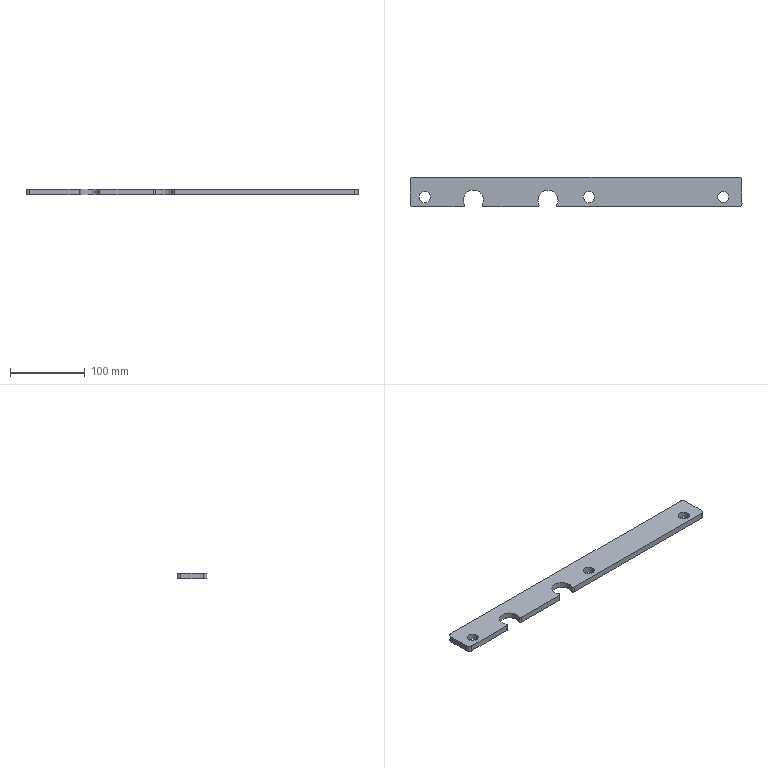Part | SolidWorks | features Fillet 1, FlatPattern 1, SMBaseFlange 1, SheetMetal 1 | 1 solid | 30 faces | box 445.22 x 40 x 8 mm | volume 129798 mm3 | cylinder 22 | plane 8 | commonest cylinder face diameters 4 x6 15 x6 27 x6 10 x4
STEP:
#1=CARTESIAN_POINT('',(-35.671,12.,8.));
#2=VERTEX_POINT('',#1);
#3=CARTESIAN_POINT('',(-33.671,10.,8.));
#4=VERTEX_POINT('',#3);
#5=CARTESIAN_POINT('',(-33.671,12.,8.));
#6=DIRECTION('',(0.,0.,1.));
#7=DIRECTION('',(1.,0.,0.));
#8=AXIS2_PLACEMENT_3D('',#5,#6,#7);
#9=CIRCLE('',#8,2.);
#10=EDGE_CURVE('',#2,#4,#9,.T.);
#11=ORIENTED_EDGE('',*,*,#10,.F.);
#12=CARTESIAN_POINT('',(-35.671,12.,0.));
#13=VERTEX_POINT('',#12);
#14=CARTESIAN_POINT('',(-35.671,12.,8.));
#15=DIRECTION('',(0.,0.,-1.));
#16=VECTOR('',#15,1000.);
#17=LINE('',#14,#16);
#18=EDGE_CURVE('',#2,#13,#17,.T.);
#19=ORIENTED_EDGE('',*,*,#18,.T.);
#20=CARTESIAN_POINT('',(-33.671,10.,0.));
#21=VERTEX_POINT('',#20);
#22=CARTESIAN_POINT('',(-33.671,12.,0.));
#23=DIRECTION('',(0.,0.,-1.));
#24=DIRECTION('',(1.,0.,0.));
#25=AXIS2_PLACEMENT_3D('',#22,#23,#24);
#26=CIRCLE('',#25,2.);
#27=EDGE_CURVE('',#21,#13,#26,.T.);
#28=ORIENTED_EDGE('',*,*,#27,.F.);
#29=CARTESIAN_POINT('',(-33.671,10.,8.));
#30=DIRECTION('',(0.,0.,-1.));
#31=VECTOR('',#30,1000.);
#32=LINE('',#29,#31);
#33=EDGE_CURVE('',#4,#21,#32,.T.);
#34=ORIENTED_EDGE('',*,*,#33,.F.);
#35=EDGE_LOOP('',(#11,#19,#28,#34));
#36=FACE_OUTER_BOUND('',#35,.T.);
#37=CARTESIAN_POINT('',(-33.671,12.,8.));
#38=DIRECTION('',(0.,0.,-1.));
#39=DIRECTION('',(-1.,0.,0.));
#40=AXIS2_PLACEMENT_3D('',#37,#38,#39);
#41=CYLINDRICAL_SURFACE('',#40,2.);
#42=ADVANCED_FACE('',(#36),#41,.T.);
#43=CARTESIAN_POINT('',(64.329,12.,8.));
#44=VERTEX_POINT('',#43);
#45=CARTESIAN_POINT('',(66.329,10.,8.));
#46=VERTEX_POINT('',#45);
#47=CARTESIAN_POINT('',(66.329,12.,8.));
#48=DIRECTION('',(0.,0.,1.));
#49=DIRECTION('',(1.,0.,0.));
#50=AXIS2_PLACEMENT_3D('',#47,#48,#49);
#51=CIRCLE('',#50,2.);
#52=EDGE_CURVE('',#44,#46,#51,.T.);
#53=ORIENTED_EDGE('',*,*,#52,.F.);
#54=CARTESIAN_POINT('',(64.329,12.,0.));
#55=VERTEX_POINT('',#54);
#56=CARTESIAN_POINT('',(64.329,12.,8.));
#57=DIRECTION('',(0.,0.,-1.));
#58=VECTOR('',#57,1000.);
#59=LINE('',#56,#58);
#60=EDGE_CURVE('',#44,#55,#59,.T.);
#61=ORIENTED_EDGE('',*,*,#60,.T.);
#62=CARTESIAN_POINT('',(66.329,10.,0.));
#63=VERTEX_POINT('',#62);
#64=CARTESIAN_POINT('',(66.329,12.,0.));
#65=DIRECTION('',(0.,0.,-1.));
#66=DIRECTION('',(1.,0.,0.));
#67=AXIS2_PLACEMENT_3D('',#64,#65,#66);
#68=CIRCLE('',#67,2.);
#69=EDGE_CURVE('',#63,#55,#68,.T.);
#70=ORIENTED_EDGE('',*,*,#69,.F.);
#71=CARTESIAN_POINT('',(66.329,10.,8.));
#72=DIRECTION('',(0.,0.,-1.));
#73=VECTOR('',#72,1000.);
#74=LINE('',#71,#73);
#75=EDGE_CURVE('',#46,#63,#74,.T.);
#76=ORIENTED_EDGE('',*,*,#75,.F.);
#77=EDGE_LOOP('',(#53,#61,#70,#76));
#78=FACE_OUTER_BOUND('',#77,.T.);
#79=CARTESIAN_POINT('',(66.329,12.,8.));
#80=DIRECTION('',(0.,0.,-1.));
#81=DIRECTION('',(-1.,0.,0.));
#82=AXIS2_PLACEMENT_3D('',#79,#80,#81);
#83=CYLINDRICAL_SURFACE('',#82,2.);
#84=ADVANCED_FACE('',(#78),#83,.T.);
#85=CARTESIAN_POINT('',(279.991,23.188,8.));
#86=VERTEX_POINT('',#85);
#87=CARTESIAN_POINT('',(294.991,23.188,8.));
#88=VERTEX_POINT('',#87);
#89=CARTESIAN_POINT('',(287.491,23.188,8.));
#90=DIRECTION('',(0.,0.,1.));
#91=DIRECTION('',(1.,0.,0.));
#92=AXIS2_PLACEMENT_3D('',#89,#90,#91);
#93=CIRCLE('',#92,7.5);
#94=EDGE_CURVE('',#86,#88,#93,.T.);
#95=ORIENTED_EDGE('',*,*,#94,.T.);
#96=CARTESIAN_POINT('',(294.991,23.188,0.));
#97=VERTEX_POINT('',#96);
#98=CARTESIAN_POINT('',(294.991,23.188,8.));
#99=DIRECTION('',(0.,0.,-1.));
#100=VECTOR('',#99,1000.);
#101=LINE('',#98,#100);
#102=EDGE_CURVE('',#88,#97,#101,.T.);
#103=ORIENTED_EDGE('',*,*,#102,.T.);
#104=CARTESIAN_POINT('',(279.991,23.188,0.));
#105=VERTEX_POINT('',#104);
#106=CARTESIAN_POINT('',(287.491,23.188,0.));
#107=DIRECTION('',(0.,0.,1.));
#108=DIRECTION('',(1.,0.,0.));
#109=AXIS2_PLACEMENT_3D('',#106,#107,#108);
#110=CIRCLE('',#109,7.5);
#111=EDGE_CURVE('',#105,#97,#110,.T.);
#112=ORIENTED_EDGE('',*,*,#111,.F.);
#113=CARTESIAN_POINT('',(279.991,23.188,8.));
#114=DIRECTION('',(0.,0.,-1.));
#115=VECTOR('',#114,1000.);
#116=LINE('',#113,#115);
#117=EDGE_CURVE('',#86,#105,#116,.T.);
#118=ORIENTED_EDGE('',*,*,#117,.F.);
#119=EDGE_LOOP('',(#95,#103,#112,#118));
#120=FACE_OUTER_BOUND('',#119,.T.);
#121=CARTESIAN_POINT('',(287.491,23.188,8.));
#122=DIRECTION('',(0.,0.,-1.));
#123=DIRECTION('',(-1.,0.,0.));
#124=AXIS2_PLACEMENT_3D('',#121,#122,#123);
#125=CYLINDRICAL_SURFACE('',#124,7.5);
#126=ADVANCED_FACE('',(#120),#125,.F.);
#127=CARTESIAN_POINT('',(100.,23.,8.));
#128=VERTEX_POINT('',#127);
#129=CARTESIAN_POINT('',(115.,23.,8.));
#130=VERTEX_POINT('',#129);
#131=CARTESIAN_POINT('',(107.5,23.,8.));
#132=DIRECTION('',(0.,0.,1.));
#133=DIRECTION('',(1.,0.,0.));
#134=AXIS2_PLACEMENT_3D('',#131,#132,#133);
#135=CIRCLE('',#134,7.5);
#136=EDGE_CURVE('',#128,#130,#135,.T.);
#137=ORIENTED_EDGE('',*,*,#136,.T.);
#138=CARTESIAN_POINT('',(115.,23.,0.));
#139=VERTEX_POINT('',#138);
#140=CARTESIAN_POINT('',(115.,23.,8.));
#141=DIRECTION('',(0.,0.,-1.));
#142=VECTOR('',#141,1000.);
#143=LINE('',#140,#142);
#144=EDGE_CURVE('',#130,#139,#143,.T.);
#145=ORIENTED_EDGE('',*,*,#144,.T.);
#146=CARTESIAN_POINT('',(100.,23.,0.));
#147=VERTEX_POINT('',#146);
#148=CARTESIAN_POINT('',(107.5,23.,0.));
#149=DIRECTION('',(0.,0.,1.));
#150=DIRECTION('',(1.,0.,0.));
#151=AXIS2_PLACEMENT_3D('',#148,#149,#150);
#152=CIRCLE('',#151,7.5);
#153=EDGE_CURVE('',#147,#139,#152,.T.);
#154=ORIENTED_EDGE('',*,*,#153,.F.);
#155=CARTESIAN_POINT('',(100.,23.,8.));
#156=DIRECTION('',(0.,0.,-1.));
#157=VECTOR('',#156,1000.);
#158=LINE('',#155,#157);
#159=EDGE_CURVE('',#128,#147,#158,.T.);
#160=ORIENTED_EDGE('',*,*,#159,.F.);
#161=EDGE_LOOP('',(#137,#145,#154,#160));
#162=FACE_OUTER_BOUND('',#161,.T.);
#163=CARTESIAN_POINT('',(107.5,23.,8.));
#164=DIRECTION('',(0.,0.,-1.));
#165=DIRECTION('',(-1.,0.,0.));
#166=AXIS2_PLACEMENT_3D('',#163,#164,#165);
#167=CYLINDRICAL_SURFACE('',#166,7.5);
#168=ADVANCED_FACE('',(#162),#167,.F.);
#169=CARTESIAN_POINT('',(-120.,23.,8.));
#170=VERTEX_POINT('',#169);
#171=CARTESIAN_POINT('',(-105.,23.,8.));
#172=VERTEX_POINT('',#171);
#173=CARTESIAN_POINT('',(-112.5,23.,8.));
#174=DIRECTION('',(0.,0.,1.));
#175=DIRECTION('',(1.,0.,0.));
#176=AXIS2_PLACEMENT_3D('',#173,#174,#175);
#177=CIRCLE('',#176,7.5);
#178=EDGE_CURVE('',#170,#172,#177,.T.);
#179=ORIENTED_EDGE('',*,*,#178,.T.);
#180=CARTESIAN_POINT('',(-105.,23.,0.));
#181=VERTEX_POINT('',#180);
#182=CARTESIAN_POINT('',(-105.,23.,8.));
#183=DIRECTION('',(0.,0.,-1.));
#184=VECTOR('',#183,1000.);
#185=LINE('',#182,#184);
#186=EDGE_CURVE('',#172,#181,#185,.T.);
#187=ORIENTED_EDGE('',*,*,#186,.T.);
#188=CARTESIAN_POINT('',(-120.,23.,0.));
#189=VERTEX_POINT('',#188);
#190=CARTESIAN_POINT('',(-112.5,23.,0.));
#191=DIRECTION('',(0.,0.,1.));
#192=DIRECTION('',(1.,0.,0.));
#193=AXIS2_PLACEMENT_3D('',#190,#191,#192);
#194=CIRCLE('',#193,7.5);
#195=EDGE_CURVE('',#189,#181,#194,.T.);
#196=ORIENTED_EDGE('',*,*,#195,.F.);
#197=CARTESIAN_POINT('',(-120.,23.,8.));
#198=DIRECTION('',(0.,0.,-1.));
#199=VECTOR('',#198,1000.);
#200=LINE('',#197,#199);
#201=EDGE_CURVE('',#170,#189,#200,.T.);
#202=ORIENTED_EDGE('',*,*,#201,.F.);
#203=EDGE_LOOP('',(#179,#187,#196,#202));
#204=FACE_OUTER_BOUND('',#203,.T.);
#205=CARTESIAN_POINT('',(-112.5,23.,8.));
#206=DIRECTION('',(0.,0.,-1.));
#207=DIRECTION('',(-1.,0.,0.));
#208=AXIS2_PLACEMENT_3D('',#205,#206,#207);
#209=CYLINDRICAL_SURFACE('',#208,7.5);
#210=ADVANCED_FACE('',(#204),#209,.F.);
#211=CARTESIAN_POINT('',(66.,19.,8.));
#212=VERTEX_POINT('',#211);
#213=CARTESIAN_POINT('',(64.545,12.903,8.));
#214=VERTEX_POINT('',#213);
#215=CARTESIAN_POINT('',(52.5,19.,8.));
#216=DIRECTION('',(0.,0.,-1.));
#217=DIRECTION('',(1.,0.,0.));
#218=AXIS2_PLACEMENT_3D('',#215,#216,#217);
#219=CIRCLE('',#218,13.5);
#220=EDGE_CURVE('',#212,#214,#219,.T.);
#221=ORIENTED_EDGE('',*,*,#220,.F.);
#222=CARTESIAN_POINT('',(66.,19.,0.));
#223=VERTEX_POINT('',#222);
#224=CARTESIAN_POINT('',(66.,19.,8.));
#225=DIRECTION('',(0.,0.,-1.));
#226=VECTOR('',#225,1000.);
#227=LINE('',#224,#226);
#228=EDGE_CURVE('',#212,#223,#227,.T.);
#229=ORIENTED_EDGE('',*,*,#228,.T.);
#230=CARTESIAN_POINT('',(64.545,12.903,0.));
#231=VERTEX_POINT('',#230);
#232=CARTESIAN_POINT('',(52.5,19.,0.));
#233=DIRECTION('',(0.,0.,-1.));
#234=DIRECTION('',(1.,0.,0.));
#235=AXIS2_PLACEMENT_3D('',#232,#233,#234);
#236=CIRCLE('',#235,13.5);
#237=EDGE_CURVE('',#223,#231,#236,.T.);
#238=ORIENTED_EDGE('',*,*,#237,.T.);
#239=CARTESIAN_POINT('',(64.545,12.903,8.));
#240=DIRECTION('',(0.,0.,1.));
#241=VECTOR('',#240,1000.);
#242=LINE('',#239,#241);
#243=EDGE_CURVE('',#231,#214,#242,.T.);
#244=ORIENTED_EDGE('',*,*,#243,.T.);
#245=EDGE_LOOP('',(#221,#229,#238,#244));
#246=FACE_OUTER_BOUND('',#245,.T.);
#247=CARTESIAN_POINT('',(52.5,19.,8.));
#248=DIRECTION('',(0.,0.,-1.));
#249=DIRECTION('',(-1.,0.,0.));
#250=AXIS2_PLACEMENT_3D('',#247,#248,#249);
#251=CYLINDRICAL_SURFACE('',#250,13.5);
#252=ADVANCED_FACE('',(#246),#251,.F.);
#253=ORIENTED_EDGE('',*,*,#228,.F.);
#254=CARTESIAN_POINT('',(39.,19.,8.));
#255=VERTEX_POINT('',#254);
#256=CARTESIAN_POINT('',(52.5,19.,8.));
#257=DIRECTION('',(0.,0.,-1.));
#258=DIRECTION('',(1.,0.,0.));
#259=AXIS2_PLACEMENT_3D('',#256,#257,#258);
#260=CIRCLE('',#259,13.5);
#261=EDGE_CURVE('',#255,#212,#260,.T.);
#262=ORIENTED_EDGE('',*,*,#261,.F.);
#263=CARTESIAN_POINT('',(39.,19.,0.));
#264=VERTEX_POINT('',#263);
#265=CARTESIAN_POINT('',(39.,19.,8.));
#266=DIRECTION('',(0.,0.,-1.));
#267=VECTOR('',#266,1000.);
#268=LINE('',#265,#267);
#269=EDGE_CURVE('',#255,#264,#268,.T.);
#270=ORIENTED_EDGE('',*,*,#269,.T.);
#271=CARTESIAN_POINT('',(52.5,19.,0.));
#272=DIRECTION('',(0.,0.,-1.));
#273=DIRECTION('',(1.,0.,0.));
#274=AXIS2_PLACEMENT_3D('',#271,#272,#273);
#275=CIRCLE('',#274,13.5);
#276=EDGE_CURVE('',#264,#223,#275,.T.);
#277=ORIENTED_EDGE('',*,*,#276,.T.);
#278=EDGE_LOOP('',(#253,#262,#270,#277));
#279=FACE_OUTER_BOUND('',#278,.T.);
#280=CARTESIAN_POINT('',(52.5,19.,8.));
#281=DIRECTION('',(0.,0.,-1.));
#282=DIRECTION('',(-1.,0.,0.));
#283=AXIS2_PLACEMENT_3D('',#280,#281,#282);
#284=CYLINDRICAL_SURFACE('',#283,13.5);
#285=ADVANCED_FACE('',(#279),#284,.F.);
#286=CARTESIAN_POINT('',(-34.,19.,8.));
#287=VERTEX_POINT('',#286);
#288=CARTESIAN_POINT('',(-35.455,12.903,8.));
#289=VERTEX_POINT('',#288);
#290=CARTESIAN_POINT('',(-47.5,19.,8.));
#291=DIRECTION('',(0.,0.,-1.));
#292=DIRECTION('',(1.,0.,0.));
#293=AXIS2_PLACEMENT_3D('',#290,#291,#292);
#294=CIRCLE('',#293,13.5);
#295=EDGE_CURVE('',#287,#289,#294,.T.);
#296=ORIENTED_EDGE('',*,*,#295,.F.);
#297=CARTESIAN_POINT('',(-34.,19.,0.));
#298=VERTEX_POINT('',#297);
#299=CARTESIAN_POINT('',(-34.,19.,8.));
#300=DIRECTION('',(0.,0.,-1.));
#301=VECTOR('',#300,1000.);
#302=LINE('',#299,#301);
#303=EDGE_CURVE('',#287,#298,#302,.T.);
#304=ORIENTED_EDGE('',*,*,#303,.T.);
#305=CARTESIAN_POINT('',(-35.455,12.903,0.));
#306=VERTEX_POINT('',#305);
#307=CARTESIAN_POINT('',(-47.5,19.,0.));
#308=DIRECTION('',(0.,0.,-1.));
#309=DIRECTION('',(1.,0.,0.));
#310=AXIS2_PLACEMENT_3D('',#307,#308,#309);
#311=CIRCLE('',#310,13.5);
#312=EDGE_CURVE('',#298,#306,#311,.T.);
#313=ORIENTED_EDGE('',*,*,#312,.T.);
#314=CARTESIAN_POINT('',(-35.455,12.903,8.));
#315=DIRECTION('',(0.,0.,1.));
#316=VECTOR('',#315,1000.);
#317=LINE('',#314,#316);
#318=EDGE_CURVE('',#306,#289,#317,.T.);
#319=ORIENTED_EDGE('',*,*,#318,.T.);
#320=EDGE_LOOP('',(#296,#304,#313,#319));
#321=FACE_OUTER_BOUND('',#320,.T.);
#322=CARTESIAN_POINT('',(-47.5,19.,8.));
#323=DIRECTION('',(0.,0.,-1.));
#324=DIRECTION('',(-1.,0.,0.));
#325=AXIS2_PLACEMENT_3D('',#322,#323,#324);
#326=CYLINDRICAL_SURFACE('',#325,13.5);
#327=ADVANCED_FACE('',(#321),#326,.F.);
#328=ORIENTED_EDGE('',*,*,#303,.F.);
#329=CARTESIAN_POINT('',(-61.,19.,8.));
#330=VERTEX_POINT('',#329);
#331=CARTESIAN_POINT('',(-47.5,19.,8.));
#332=DIRECTION('',(0.,0.,-1.));
#333=DIRECTION('',(1.,0.,0.));
#334=AXIS2_PLACEMENT_3D('',#331,#332,#333);
#335=CIRCLE('',#334,13.5);
#336=EDGE_CURVE('',#330,#287,#335,.T.);
#337=ORIENTED_EDGE('',*,*,#336,.F.);
#338=CARTESIAN_POINT('',(-61.,19.,0.));
#339=VERTEX_POINT('',#338);
#340=CARTESIAN_POINT('',(-61.,19.,8.));
#341=DIRECTION('',(0.,0.,-1.));
#342=VECTOR('',#341,1000.);
#343=LINE('',#340,#342);
#344=EDGE_CURVE('',#330,#339,#343,.T.);
#345=ORIENTED_EDGE('',*,*,#344,.T.);
#346=CARTESIAN_POINT('',(-47.5,19.,0.));
#347=DIRECTION('',(0.,0.,-1.));
#348=DIRECTION('',(1.,0.,0.));
#349=AXIS2_PLACEMENT_3D('',#346,#347,#348);
#350=CIRCLE('',#349,13.5);
#351=EDGE_CURVE('',#339,#298,#350,.T.);
#352=ORIENTED_EDGE('',*,*,#351,.T.);
#353=EDGE_LOOP('',(#328,#337,#345,#352));
#354=FACE_OUTER_BOUND('',#353,.T.);
#355=CARTESIAN_POINT('',(-47.5,19.,8.));
#356=DIRECTION('',(0.,0.,-1.));
#357=DIRECTION('',(-1.,0.,0.));
#358=AXIS2_PLACEMENT_3D('',#355,#356,#357);
#359=CYLINDRICAL_SURFACE('',#358,13.5);
#360=ADVANCED_FACE('',(#354),#359,.F.);
#361=ORIENTED_EDGE('',*,*,#136,.F.);
#362=CARTESIAN_POINT('',(107.5,23.,8.));
#363=DIRECTION('',(0.,0.,1.));
#364=DIRECTION('',(1.,0.,0.));
#365=AXIS2_PLACEMENT_3D('',#362,#363,#364);
#366=CIRCLE('',#365,7.5);
#367=EDGE_CURVE('',#130,#128,#366,.T.);
#368=ORIENTED_EDGE('',*,*,#367,.F.);
#369=EDGE_LOOP('',(#361,#368));
#370=FACE_BOUND('',#369,.T.);
#371=CARTESIAN_POINT('',(38.671,10.,8.));
#372=VERTEX_POINT('',#371);
#373=CARTESIAN_POINT('',(42.438,10.,8.));
#374=DIRECTION('',(1.,0.,0.));
#375=VECTOR('',#374,1000.);
#376=LINE('',#373,#375);
#377=EDGE_CURVE('',#4,#372,#376,.T.);
#378=ORIENTED_EDGE('',*,*,#377,.T.);
#379=CARTESIAN_POINT('',(40.455,12.903,8.));
#380=VERTEX_POINT('',#379);
#381=CARTESIAN_POINT('',(38.671,12.,8.));
#382=DIRECTION('',(0.,0.,1.));
#383=DIRECTION('',(1.,0.,0.));
#384=AXIS2_PLACEMENT_3D('',#381,#382,#383);
#385=CIRCLE('',#384,2.);
#386=EDGE_CURVE('',#372,#380,#385,.T.);
#387=ORIENTED_EDGE('',*,*,#386,.T.);
#388=CARTESIAN_POINT('',(52.5,19.,8.));
#389=DIRECTION('',(0.,0.,-1.));
#390=DIRECTION('',(1.,0.,0.));
#391=AXIS2_PLACEMENT_3D('',#388,#389,#390);
#392=CIRCLE('',#391,13.5);
#393=EDGE_CURVE('',#380,#255,#392,.T.);
#394=ORIENTED_EDGE('',*,*,#393,.T.);
#395=ORIENTED_EDGE('',*,*,#261,.T.);
#396=ORIENTED_EDGE('',*,*,#220,.T.);
#397=CARTESIAN_POINT('',(66.329,12.,8.));
#398=DIRECTION('',(0.,0.,1.));
#399=DIRECTION('',(1.,0.,0.));
#400=AXIS2_PLACEMENT_3D('',#397,#398,#399);
#401=CIRCLE('',#400,2.);
#402=EDGE_CURVE('',#214,#44,#401,.T.);
#403=ORIENTED_EDGE('',*,*,#402,.T.);
#404=ORIENTED_EDGE('',*,*,#52,.T.);
#405=CARTESIAN_POINT('',(307.72,10.,8.));
#406=VERTEX_POINT('',#405);
#407=CARTESIAN_POINT('',(307.72,10.,8.));
#408=DIRECTION('',(1.,0.,0.));
#409=VECTOR('',#408,1000.);
#410=LINE('',#407,#409);
#411=EDGE_CURVE('',#46,#406,#410,.T.);
#412=ORIENTED_EDGE('',*,*,#411,.T.);
#413=CARTESIAN_POINT('',(312.72,15.01,8.));
#414=VERTEX_POINT('',#413);
#415=CARTESIAN_POINT('',(307.72,15.,8.));
#416=DIRECTION('',(0.,0.,1.));
#417=DIRECTION('',(-1.,0.,0.));
#418=AXIS2_PLACEMENT_3D('',#415,#416,#417);
#419=CIRCLE('',#418,5.);
#420=EDGE_CURVE('',#406,#414,#419,.T.);
#421=ORIENTED_EDGE('',*,*,#420,.T.);
#422=CARTESIAN_POINT('',(312.661,45.01,8.));
#423=VERTEX_POINT('',#422);
#424=CARTESIAN_POINT('',(312.661,45.01,8.));
#425=DIRECTION('',(-0.001974,1.,0.));
#426=VECTOR('',#425,1000.);
#427=LINE('',#424,#426);
#428=EDGE_CURVE('',#414,#423,#427,.T.);
#429=ORIENTED_EDGE('',*,*,#428,.T.);
#430=CARTESIAN_POINT('',(307.661,50.,8.));
#431=VERTEX_POINT('',#430);
#432=CARTESIAN_POINT('',(307.661,45.,8.));
#433=DIRECTION('',(0.,0.,1.));
#434=DIRECTION('',(-1.,0.,0.));
#435=AXIS2_PLACEMENT_3D('',#432,#433,#434);
#436=CIRCLE('',#435,5.);
#437=EDGE_CURVE('',#423,#431,#436,.T.);
#438=ORIENTED_EDGE('',*,*,#437,.T.);
#439=CARTESIAN_POINT('',(-127.5,50.,8.));
#440=VERTEX_POINT('',#439);
#441=CARTESIAN_POINT('',(-127.5,50.,8.));
#442=DIRECTION('',(-1.,0.,0.));
#443=VECTOR('',#442,1000.);
#444=LINE('',#441,#443);
#445=EDGE_CURVE('',#431,#440,#444,.T.);
#446=ORIENTED_EDGE('',*,*,#445,.T.);
#447=CARTESIAN_POINT('',(-132.5,45.,8.));
#448=VERTEX_POINT('',#447);
#449=CARTESIAN_POINT('',(-127.5,45.,8.));
#450=DIRECTION('',(0.,0.,1.));
#451=DIRECTION('',(-1.,0.,0.));
#452=AXIS2_PLACEMENT_3D('',#449,#450,#451);
#453=CIRCLE('',#452,5.);
#454=EDGE_CURVE('',#440,#448,#453,.T.);
#455=ORIENTED_EDGE('',*,*,#454,.T.);
#456=CARTESIAN_POINT('',(-132.5,15.,8.));
#457=VERTEX_POINT('',#456);
#458=CARTESIAN_POINT('',(-132.5,15.,8.));
#459=DIRECTION('',(0.,-1.,0.));
#460=VECTOR('',#459,1000.);
#461=LINE('',#458,#460);
#462=EDGE_CURVE('',#448,#457,#461,.T.);
#463=ORIENTED_EDGE('',*,*,#462,.T.);
#464=CARTESIAN_POINT('',(-127.5,10.,8.));
#465=VERTEX_POINT('',#464);
#466=CARTESIAN_POINT('',(-127.5,15.,8.));
#467=DIRECTION('',(0.,0.,1.));
#468=DIRECTION('',(1.,0.,0.));
#469=AXIS2_PLACEMENT_3D('',#466,#467,#468);
#470=CIRCLE('',#469,5.);
#471=EDGE_CURVE('',#457,#465,#470,.T.);
#472=ORIENTED_EDGE('',*,*,#471,.T.);
#473=CARTESIAN_POINT('',(-61.329,10.,8.));
#474=VERTEX_POINT('',#473);
#475=CARTESIAN_POINT('',(-57.562,10.,8.));
#476=DIRECTION('',(1.,0.,0.));
#477=VECTOR('',#476,1000.);
#478=LINE('',#475,#477);
#479=EDGE_CURVE('',#465,#474,#478,.T.);
#480=ORIENTED_EDGE('',*,*,#479,.T.);
#481=CARTESIAN_POINT('',(-59.545,12.903,8.));
#482=VERTEX_POINT('',#481);
#483=CARTESIAN_POINT('',(-61.329,12.,8.));
#484=DIRECTION('',(0.,0.,1.));
#485=DIRECTION('',(1.,0.,0.));
#486=AXIS2_PLACEMENT_3D('',#483,#484,#485);
#487=CIRCLE('',#486,2.);
#488=EDGE_CURVE('',#474,#482,#487,.T.);
#489=ORIENTED_EDGE('',*,*,#488,.T.);
#490=CARTESIAN_POINT('',(-47.5,19.,8.));
#491=DIRECTION('',(0.,0.,-1.));
#492=DIRECTION('',(1.,0.,0.));
#493=AXIS2_PLACEMENT_3D('',#490,#491,#492);
#494=CIRCLE('',#493,13.5);
#495=EDGE_CURVE('',#482,#330,#494,.T.);
#496=ORIENTED_EDGE('',*,*,#495,.T.);
#497=ORIENTED_EDGE('',*,*,#336,.T.);
#498=ORIENTED_EDGE('',*,*,#295,.T.);
#499=CARTESIAN_POINT('',(-33.671,12.,8.));
#500=DIRECTION('',(0.,0.,1.));
#501=DIRECTION('',(1.,0.,0.));
#502=AXIS2_PLACEMENT_3D('',#499,#500,#501);
#503=CIRCLE('',#502,2.);
#504=EDGE_CURVE('',#289,#2,#503,.T.);
#505=ORIENTED_EDGE('',*,*,#504,.T.);
#506=ORIENTED_EDGE('',*,*,#10,.T.);
#507=EDGE_LOOP('',(#378,#387,#394,#395,#396,#403,#404,#412,#421,#429,#438,#446,#455,#463,#472,#480,#489,#496,#497,#498,#505,#506));
#508=FACE_OUTER_BOUND('',#507,.T.);
#509=ORIENTED_EDGE('',*,*,#178,.F.);
#510=CARTESIAN_POINT('',(-112.5,23.,8.));
#511=DIRECTION('',(0.,0.,1.));
#512=DIRECTION('',(1.,0.,0.));
#513=AXIS2_PLACEMENT_3D('',#510,#511,#512);
#514=CIRCLE('',#513,7.5);
#515=EDGE_CURVE('',#172,#170,#514,.T.);
#516=ORIENTED_EDGE('',*,*,#515,.F.);
#517=EDGE_LOOP('',(#509,#516));
#518=FACE_BOUND('',#517,.T.);
#519=ORIENTED_EDGE('',*,*,#94,.F.);
#520=CARTESIAN_POINT('',(287.491,23.188,8.));
#521=DIRECTION('',(0.,0.,1.));
#522=DIRECTION('',(1.,0.,0.));
#523=AXIS2_PLACEMENT_3D('',#520,#521,#522);
#524=CIRCLE('',#523,7.5);
#525=EDGE_CURVE('',#88,#86,#524,.T.);
#526=ORIENTED_EDGE('',*,*,#525,.F.);
#527=EDGE_LOOP('',(#519,#526));
#528=FACE_BOUND('',#527,.T.);
#529=CARTESIAN_POINT('',(-47.5,19.,8.));
#530=DIRECTION('',(0.,0.,1.));
#531=DIRECTION('',(1.,0.,0.));
#532=AXIS2_PLACEMENT_3D('',#529,#530,#531);
#533=PLANE('',#532);
#534=ADVANCED_FACE('',(#370,#508,#518,#528),#533,.T.);
#535=CARTESIAN_POINT('',(40.455,12.903,0.));
#536=VERTEX_POINT('',#535);
#537=CARTESIAN_POINT('',(52.5,19.,0.));
#538=DIRECTION('',(0.,0.,-1.));
#539=DIRECTION('',(1.,0.,0.));
#540=AXIS2_PLACEMENT_3D('',#537,#538,#539);
#541=CIRCLE('',#540,13.5);
#542=EDGE_CURVE('',#536,#264,#541,.T.);
#543=ORIENTED_EDGE('',*,*,#542,.F.);
#544=CARTESIAN_POINT('',(38.671,10.,0.));
#545=VERTEX_POINT('',#544);
#546=CARTESIAN_POINT('',(38.671,12.,0.));
#547=DIRECTION('',(0.,0.,-1.));
#548=DIRECTION('',(1.,0.,0.));
#549=AXIS2_PLACEMENT_3D('',#546,#547,#548);
#550=CIRCLE('',#549,2.);
#551=EDGE_CURVE('',#536,#545,#550,.T.);
#552=ORIENTED_EDGE('',*,*,#551,.T.);
#553=CARTESIAN_POINT('',(42.438,10.,0.));
#554=DIRECTION('',(1.,0.,0.));
#555=VECTOR('',#554,1000.);
#556=LINE('',#553,#555);
#557=EDGE_CURVE('',#21,#545,#556,.T.);
#558=ORIENTED_EDGE('',*,*,#557,.F.);
#559=ORIENTED_EDGE('',*,*,#27,.T.);
#560=CARTESIAN_POINT('',(-33.671,12.,0.));
#561=DIRECTION('',(0.,0.,-1.));
#562=DIRECTION('',(1.,0.,0.));
#563=AXIS2_PLACEMENT_3D('',#560,#561,#562);
#564=CIRCLE('',#563,2.);
#565=EDGE_CURVE('',#13,#306,#564,.T.);
#566=ORIENTED_EDGE('',*,*,#565,.T.);
#567=ORIENTED_EDGE('',*,*,#312,.F.);
#568=ORIENTED_EDGE('',*,*,#351,.F.);
#569=CARTESIAN_POINT('',(-59.545,12.903,0.));
#570=VERTEX_POINT('',#569);
#571=CARTESIAN_POINT('',(-47.5,19.,0.));
#572=DIRECTION('',(0.,0.,-1.));
#573=DIRECTION('',(1.,0.,0.));
#574=AXIS2_PLACEMENT_3D('',#571,#572,#573);
#575=CIRCLE('',#574,13.5);
#576=EDGE_CURVE('',#570,#339,#575,.T.);
#577=ORIENTED_EDGE('',*,*,#576,.F.);
#578=CARTESIAN_POINT('',(-61.329,10.,0.));
#579=VERTEX_POINT('',#578);
#580=CARTESIAN_POINT('',(-61.329,12.,0.));
#581=DIRECTION('',(0.,0.,-1.));
#582=DIRECTION('',(1.,0.,0.));
#583=AXIS2_PLACEMENT_3D('',#580,#581,#582);
#584=CIRCLE('',#583,2.);
#585=EDGE_CURVE('',#570,#579,#584,.T.);
#586=ORIENTED_EDGE('',*,*,#585,.T.);
#587=CARTESIAN_POINT('',(-127.5,10.,0.));
#588=VERTEX_POINT('',#587);
#589=CARTESIAN_POINT('',(-57.562,10.,0.));
#590=DIRECTION('',(1.,0.,0.));
#591=VECTOR('',#590,1000.);
#592=LINE('',#589,#591);
#593=EDGE_CURVE('',#588,#579,#592,.T.);
#594=ORIENTED_EDGE('',*,*,#593,.F.);
#595=CARTESIAN_POINT('',(-132.5,15.,0.));
#596=VERTEX_POINT('',#595);
#597=CARTESIAN_POINT('',(-127.5,15.,0.));
#598=DIRECTION('',(0.,0.,1.));
#599=DIRECTION('',(1.,0.,0.));
#600=AXIS2_PLACEMENT_3D('',#597,#598,#599);
#601=CIRCLE('',#600,5.);
#602=EDGE_CURVE('',#596,#588,#601,.T.);
#603=ORIENTED_EDGE('',*,*,#602,.F.);
#604=CARTESIAN_POINT('',(-132.5,45.,0.));
#605=VERTEX_POINT('',#604);
#606=CARTESIAN_POINT('',(-132.5,15.,0.));
#607=DIRECTION('',(0.,-1.,0.));
#608=VECTOR('',#607,1000.);
#609=LINE('',#606,#608);
#610=EDGE_CURVE('',#605,#596,#609,.T.);
#611=ORIENTED_EDGE('',*,*,#610,.F.);
#612=CARTESIAN_POINT('',(-127.5,50.,0.));
#613=VERTEX_POINT('',#612);
#614=CARTESIAN_POINT('',(-127.5,45.,0.));
#615=DIRECTION('',(0.,0.,1.));
#616=DIRECTION('',(-1.,0.,0.));
#617=AXIS2_PLACEMENT_3D('',#614,#615,#616);
#618=CIRCLE('',#617,5.);
#619=EDGE_CURVE('',#613,#605,#618,.T.);
#620=ORIENTED_EDGE('',*,*,#619,.F.);
#621=CARTESIAN_POINT('',(307.661,50.,0.));
#622=VERTEX_POINT('',#621);
#623=CARTESIAN_POINT('',(-127.5,50.,0.));
#624=DIRECTION('',(-1.,0.,0.));
#625=VECTOR('',#624,1000.);
#626=LINE('',#623,#625);
#627=EDGE_CURVE('',#622,#613,#626,.T.);
#628=ORIENTED_EDGE('',*,*,#627,.F.);
#629=CARTESIAN_POINT('',(312.661,45.01,0.));
#630=VERTEX_POINT('',#629);
#631=CARTESIAN_POINT('',(307.661,45.,0.));
#632=DIRECTION('',(0.,0.,1.));
#633=DIRECTION('',(-1.,0.,0.));
#634=AXIS2_PLACEMENT_3D('',#631,#632,#633);
#635=CIRCLE('',#634,5.);
#636=EDGE_CURVE('',#630,#622,#635,.T.);
#637=ORIENTED_EDGE('',*,*,#636,.F.);
#638=CARTESIAN_POINT('',(312.72,15.01,0.));
#639=VERTEX_POINT('',#638);
#640=CARTESIAN_POINT('',(312.661,45.01,0.));
#641=DIRECTION('',(-0.001974,1.,0.));
#642=VECTOR('',#641,1000.);
#643=LINE('',#640,#642);
#644=EDGE_CURVE('',#639,#630,#643,.T.);
#645=ORIENTED_EDGE('',*,*,#644,.F.);
#646=CARTESIAN_POINT('',(307.72,10.,0.));
#647=VERTEX_POINT('',#646);
#648=CARTESIAN_POINT('',(307.72,15.,0.));
#649=DIRECTION('',(0.,0.,1.));
#650=DIRECTION('',(-1.,0.,0.));
#651=AXIS2_PLACEMENT_3D('',#648,#649,#650);
#652=CIRCLE('',#651,5.);
#653=EDGE_CURVE('',#647,#639,#652,.T.);
#654=ORIENTED_EDGE('',*,*,#653,.F.);
#655=CARTESIAN_POINT('',(307.72,10.,0.));
#656=DIRECTION('',(1.,0.,0.));
#657=VECTOR('',#656,1000.);
#658=LINE('',#655,#657);
#659=EDGE_CURVE('',#63,#647,#658,.T.);
#660=ORIENTED_EDGE('',*,*,#659,.F.);
#661=ORIENTED_EDGE('',*,*,#69,.T.);
#662=CARTESIAN_POINT('',(66.329,12.,0.));
#663=DIRECTION('',(0.,0.,-1.));
#664=DIRECTION('',(1.,0.,0.));
#665=AXIS2_PLACEMENT_3D('',#662,#663,#664);
#666=CIRCLE('',#665,2.);
#667=EDGE_CURVE('',#55,#231,#666,.T.);
#668=ORIENTED_EDGE('',*,*,#667,.T.);
#669=ORIENTED_EDGE('',*,*,#237,.F.);
#670=ORIENTED_EDGE('',*,*,#276,.F.);
#671=EDGE_LOOP('',(#543,#552,#558,#559,#566,#567,#568,#577,#586,#594,#603,#611,#620,#628,#637,#645,#654,#660,#661,#668,#669,#670));
#672=FACE_OUTER_BOUND('',#671,.T.);
#673=ORIENTED_EDGE('',*,*,#195,.T.);
#674=CARTESIAN_POINT('',(-112.5,23.,0.));
#675=DIRECTION('',(0.,0.,1.));
#676=DIRECTION('',(1.,0.,0.));
#677=AXIS2_PLACEMENT_3D('',#674,#675,#676);
#678=CIRCLE('',#677,7.5);
#679=EDGE_CURVE('',#181,#189,#678,.T.);
#680=ORIENTED_EDGE('',*,*,#679,.T.);
#681=EDGE_LOOP('',(#673,#680));
#682=FACE_BOUND('',#681,.T.);
#683=ORIENTED_EDGE('',*,*,#153,.T.);
#684=CARTESIAN_POINT('',(107.5,23.,0.));
#685=DIRECTION('',(0.,0.,1.));
#686=DIRECTION('',(1.,0.,0.));
#687=AXIS2_PLACEMENT_3D('',#684,#685,#686);
#688=CIRCLE('',#687,7.5);
#689=EDGE_CURVE('',#139,#147,#688,.T.);
#690=ORIENTED_EDGE('',*,*,#689,.T.);
#691=EDGE_LOOP('',(#683,#690));
#692=FACE_BOUND('',#691,.T.);
#693=ORIENTED_EDGE('',*,*,#111,.T.);
#694=CARTESIAN_POINT('',(287.491,23.188,0.));
#695=DIRECTION('',(0.,0.,1.));
#696=DIRECTION('',(1.,0.,0.));
#697=AXIS2_PLACEMENT_3D('',#694,#695,#696);
#698=CIRCLE('',#697,7.5);
#699=EDGE_CURVE('',#97,#105,#698,.T.);
#700=ORIENTED_EDGE('',*,*,#699,.T.);
#701=EDGE_LOOP('',(#693,#700));
#702=FACE_BOUND('',#701,.T.);
#703=CARTESIAN_POINT('',(-47.5,19.,0.));
#704=DIRECTION('',(0.,0.,1.));
#705=DIRECTION('',(1.,0.,0.));
#706=AXIS2_PLACEMENT_3D('',#703,#704,#705);
#707=PLANE('',#706);
#708=ADVANCED_FACE('',(#672,#682,#692,#702),#707,.F.);
#709=ORIENTED_EDGE('',*,*,#344,.F.);
#710=ORIENTED_EDGE('',*,*,#495,.F.);
#711=CARTESIAN_POINT('',(-59.545,12.903,8.));
#712=DIRECTION('',(0.,0.,-1.));
#713=VECTOR('',#712,1000.);
#714=LINE('',#711,#713);
#715=EDGE_CURVE('',#482,#570,#714,.T.);
#716=ORIENTED_EDGE('',*,*,#715,.T.);
#717=ORIENTED_EDGE('',*,*,#576,.T.);
#718=EDGE_LOOP('',(#709,#710,#716,#717));
#719=FACE_OUTER_BOUND('',#718,.T.);
#720=CARTESIAN_POINT('',(-47.5,19.,8.));
#721=DIRECTION('',(0.,0.,-1.));
#722=DIRECTION('',(-1.,0.,0.));
#723=AXIS2_PLACEMENT_3D('',#720,#721,#722);
#724=CYLINDRICAL_SURFACE('',#723,13.5);
#725=ADVANCED_FACE('',(#719),#724,.F.);
#726=ORIENTED_EDGE('',*,*,#557,.T.);
#727=CARTESIAN_POINT('',(38.671,10.,8.));
#728=DIRECTION('',(0.,0.,1.));
#729=VECTOR('',#728,1000.);
#730=LINE('',#727,#729);
#731=EDGE_CURVE('',#545,#372,#730,.T.);
#732=ORIENTED_EDGE('',*,*,#731,.T.);
#733=ORIENTED_EDGE('',*,*,#377,.F.);
#734=ORIENTED_EDGE('',*,*,#33,.T.);
#735=EDGE_LOOP('',(#726,#732,#733,#734));
#736=FACE_OUTER_BOUND('',#735,.T.);
#737=CARTESIAN_POINT('',(42.438,10.,8.));
#738=DIRECTION('',(0.,1.,0.));
#739=DIRECTION('',(-1.,0.,0.));
#740=AXIS2_PLACEMENT_3D('',#737,#738,#739);
#741=PLANE('',#740);
#742=ADVANCED_FACE('',(#736),#741,.F.);
#743=ORIENTED_EDGE('',*,*,#269,.F.);
#744=ORIENTED_EDGE('',*,*,#393,.F.);
#745=CARTESIAN_POINT('',(40.455,12.903,8.));
#746=DIRECTION('',(0.,0.,-1.));
#747=VECTOR('',#746,1000.);
#748=LINE('',#745,#747);
#749=EDGE_CURVE('',#380,#536,#748,.T.);
#750=ORIENTED_EDGE('',*,*,#749,.T.);
#751=ORIENTED_EDGE('',*,*,#542,.T.);
#752=EDGE_LOOP('',(#743,#744,#750,#751));
#753=FACE_OUTER_BOUND('',#752,.T.);
#754=CARTESIAN_POINT('',(52.5,19.,8.));
#755=DIRECTION('',(0.,0.,-1.));
#756=DIRECTION('',(-1.,0.,0.));
#757=AXIS2_PLACEMENT_3D('',#754,#755,#756);
#758=CYLINDRICAL_SURFACE('',#757,13.5);
#759=ADVANCED_FACE('',(#753),#758,.F.);
#760=ORIENTED_EDGE('',*,*,#411,.F.);
#761=ORIENTED_EDGE('',*,*,#75,.T.);
#762=ORIENTED_EDGE('',*,*,#659,.T.);
#763=CARTESIAN_POINT('',(307.72,10.,8.));
#764=DIRECTION('',(0.,0.,-1.));
#765=VECTOR('',#764,1000.);
#766=LINE('',#763,#765);
#767=EDGE_CURVE('',#406,#647,#766,.T.);
#768=ORIENTED_EDGE('',*,*,#767,.F.);
#769=EDGE_LOOP('',(#760,#761,#762,#768));
#770=FACE_OUTER_BOUND('',#769,.T.);
#771=CARTESIAN_POINT('',(307.72,10.,8.));
#772=DIRECTION('',(0.,1.,0.));
#773=DIRECTION('',(-1.,0.,0.));
#774=AXIS2_PLACEMENT_3D('',#771,#772,#773);
#775=PLANE('',#774);
#776=ADVANCED_FACE('',(#770),#775,.F.);
#777=ORIENTED_EDGE('',*,*,#653,.T.);
#778=CARTESIAN_POINT('',(312.72,15.01,8.));
#779=DIRECTION('',(0.,0.,-1.));
#780=VECTOR('',#779,1000.);
#781=LINE('',#778,#780);
#782=EDGE_CURVE('',#414,#639,#781,.T.);
#783=ORIENTED_EDGE('',*,*,#782,.F.);
#784=ORIENTED_EDGE('',*,*,#420,.F.);
#785=ORIENTED_EDGE('',*,*,#767,.T.);
#786=EDGE_LOOP('',(#777,#783,#784,#785));
#787=FACE_OUTER_BOUND('',#786,.T.);
#788=CARTESIAN_POINT('',(307.72,15.,8.));
#789=DIRECTION('',(0.,0.,-1.));
#790=DIRECTION('',(-1.,0.,0.));
#791=AXIS2_PLACEMENT_3D('',#788,#789,#790);
#792=CYLINDRICAL_SURFACE('',#791,5.);
#793=ADVANCED_FACE('',(#787),#792,.T.);
#794=ORIENTED_EDGE('',*,*,#644,.T.);
#795=CARTESIAN_POINT('',(312.661,45.01,8.));
#796=DIRECTION('',(0.,0.,-1.));
#797=VECTOR('',#796,1000.);
#798=LINE('',#795,#797);
#799=EDGE_CURVE('',#423,#630,#798,.T.);
#800=ORIENTED_EDGE('',*,*,#799,.F.);
#801=ORIENTED_EDGE('',*,*,#428,.F.);
#802=ORIENTED_EDGE('',*,*,#782,.T.);
#803=EDGE_LOOP('',(#794,#800,#801,#802));
#804=FACE_OUTER_BOUND('',#803,.T.);
#805=CARTESIAN_POINT('',(312.661,45.01,8.));
#806=DIRECTION('',(-1.,-0.001974,0.));
#807=DIRECTION('',(0.001974,-1.,0.));
#808=AXIS2_PLACEMENT_3D('',#805,#806,#807);
#809=PLANE('',#808);
#810=ADVANCED_FACE('',(#804),#809,.F.);
#811=ORIENTED_EDGE('',*,*,#636,.T.);
#812=CARTESIAN_POINT('',(307.661,50.,8.));
#813=DIRECTION('',(0.,0.,-1.));
#814=VECTOR('',#813,1000.);
#815=LINE('',#812,#814);
#816=EDGE_CURVE('',#431,#622,#815,.T.);
#817=ORIENTED_EDGE('',*,*,#816,.F.);
#818=ORIENTED_EDGE('',*,*,#437,.F.);
#819=ORIENTED_EDGE('',*,*,#799,.T.);
#820=EDGE_LOOP('',(#811,#817,#818,#819));
#821=FACE_OUTER_BOUND('',#820,.T.);
#822=CARTESIAN_POINT('',(307.661,45.,8.));
#823=DIRECTION('',(0.,0.,-1.));
#824=DIRECTION('',(-1.,0.,0.));
#825=AXIS2_PLACEMENT_3D('',#822,#823,#824);
#826=CYLINDRICAL_SURFACE('',#825,5.);
#827=ADVANCED_FACE('',(#821),#826,.T.);
#828=ORIENTED_EDGE('',*,*,#627,.T.);
#829=CARTESIAN_POINT('',(-127.5,50.,8.));
#830=DIRECTION('',(0.,0.,-1.));
#831=VECTOR('',#830,1000.);
#832=LINE('',#829,#831);
#833=EDGE_CURVE('',#440,#613,#832,.T.);
#834=ORIENTED_EDGE('',*,*,#833,.F.);
#835=ORIENTED_EDGE('',*,*,#445,.F.);
#836=ORIENTED_EDGE('',*,*,#816,.T.);
#837=EDGE_LOOP('',(#828,#834,#835,#836));
#838=FACE_OUTER_BOUND('',#837,.T.);
#839=CARTESIAN_POINT('',(-127.5,50.,8.));
#840=DIRECTION('',(0.,-1.,0.));
#841=DIRECTION('',(0.,0.,-1.));
#842=AXIS2_PLACEMENT_3D('',#839,#840,#841);
#843=PLANE('',#842);
#844=ADVANCED_FACE('',(#838),#843,.F.);
#845=ORIENTED_EDGE('',*,*,#619,.T.);
#846=CARTESIAN_POINT('',(-132.5,45.,8.));
#847=DIRECTION('',(0.,0.,-1.));
#848=VECTOR('',#847,1000.);
#849=LINE('',#846,#848);
#850=EDGE_CURVE('',#448,#605,#849,.T.);
#851=ORIENTED_EDGE('',*,*,#850,.F.);
#852=ORIENTED_EDGE('',*,*,#454,.F.);
#853=ORIENTED_EDGE('',*,*,#833,.T.);
#854=EDGE_LOOP('',(#845,#851,#852,#853));
#855=FACE_OUTER_BOUND('',#854,.T.);
#856=CARTESIAN_POINT('',(-127.5,45.,8.));
#857=DIRECTION('',(0.,0.,-1.));
#858=DIRECTION('',(-1.,0.,0.));
#859=AXIS2_PLACEMENT_3D('',#856,#857,#858);
#860=CYLINDRICAL_SURFACE('',#859,5.);
#861=ADVANCED_FACE('',(#855),#860,.T.);
#862=ORIENTED_EDGE('',*,*,#610,.T.);
#863=CARTESIAN_POINT('',(-132.5,15.,8.));
#864=DIRECTION('',(0.,0.,-1.));
#865=VECTOR('',#864,1000.);
#866=LINE('',#863,#865);
#867=EDGE_CURVE('',#457,#596,#866,.T.);
#868=ORIENTED_EDGE('',*,*,#867,.F.);
#869=ORIENTED_EDGE('',*,*,#462,.F.);
#870=ORIENTED_EDGE('',*,*,#850,.T.);
#871=EDGE_LOOP('',(#862,#868,#869,#870));
#872=FACE_OUTER_BOUND('',#871,.T.);
#873=CARTESIAN_POINT('',(-132.5,15.,8.));
#874=DIRECTION('',(1.,0.,0.));
#875=DIRECTION('',(0.,0.,-1.));
#876=AXIS2_PLACEMENT_3D('',#873,#874,#875);
#877=PLANE('',#876);
#878=ADVANCED_FACE('',(#872),#877,.F.);
#879=ORIENTED_EDGE('',*,*,#602,.T.);
#880=CARTESIAN_POINT('',(-127.5,10.,8.));
#881=DIRECTION('',(0.,0.,-1.));
#882=VECTOR('',#881,1000.);
#883=LINE('',#880,#882);
#884=EDGE_CURVE('',#465,#588,#883,.T.);
#885=ORIENTED_EDGE('',*,*,#884,.F.);
#886=ORIENTED_EDGE('',*,*,#471,.F.);
#887=ORIENTED_EDGE('',*,*,#867,.T.);
#888=EDGE_LOOP('',(#879,#885,#886,#887));
#889=FACE_OUTER_BOUND('',#888,.T.);
#890=CARTESIAN_POINT('',(-127.5,15.,8.));
#891=DIRECTION('',(0.,0.,-1.));
#892=DIRECTION('',(-1.,0.,0.));
#893=AXIS2_PLACEMENT_3D('',#890,#891,#892);
#894=CYLINDRICAL_SURFACE('',#893,5.);
#895=ADVANCED_FACE('',(#889),#894,.T.);
#896=ORIENTED_EDGE('',*,*,#593,.T.);
#897=CARTESIAN_POINT('',(-61.329,10.,8.));
#898=DIRECTION('',(0.,0.,1.));
#899=VECTOR('',#898,1000.);
#900=LINE('',#897,#899);
#901=EDGE_CURVE('',#579,#474,#900,.T.);
#902=ORIENTED_EDGE('',*,*,#901,.T.);
#903=ORIENTED_EDGE('',*,*,#479,.F.);
#904=ORIENTED_EDGE('',*,*,#884,.T.);
#905=EDGE_LOOP('',(#896,#902,#903,#904));
#906=FACE_OUTER_BOUND('',#905,.T.);
#907=CARTESIAN_POINT('',(-57.562,10.,8.));
#908=DIRECTION('',(0.,1.,0.));
#909=DIRECTION('',(-1.,0.,0.));
#910=AXIS2_PLACEMENT_3D('',#907,#908,#909);
#911=PLANE('',#910);
#912=ADVANCED_FACE('',(#906),#911,.F.);
#913=ORIENTED_EDGE('',*,*,#186,.F.);
#914=ORIENTED_EDGE('',*,*,#515,.T.);
#915=ORIENTED_EDGE('',*,*,#201,.T.);
#916=ORIENTED_EDGE('',*,*,#679,.F.);
#917=EDGE_LOOP('',(#913,#914,#915,#916));
#918=FACE_OUTER_BOUND('',#917,.T.);
#919=CARTESIAN_POINT('',(-112.5,23.,8.));
#920=DIRECTION('',(0.,0.,-1.));
#921=DIRECTION('',(-1.,0.,0.));
#922=AXIS2_PLACEMENT_3D('',#919,#920,#921);
#923=CYLINDRICAL_SURFACE('',#922,7.5);
#924=ADVANCED_FACE('',(#918),#923,.F.);
#925=ORIENTED_EDGE('',*,*,#144,.F.);
#926=ORIENTED_EDGE('',*,*,#367,.T.);
#927=ORIENTED_EDGE('',*,*,#159,.T.);
#928=ORIENTED_EDGE('',*,*,#689,.F.);
#929=EDGE_LOOP('',(#925,#926,#927,#928));
#930=FACE_OUTER_BOUND('',#929,.T.);
#931=CARTESIAN_POINT('',(107.5,23.,8.));
#932=DIRECTION('',(0.,0.,-1.));
#933=DIRECTION('',(-1.,0.,0.));
#934=AXIS2_PLACEMENT_3D('',#931,#932,#933);
#935=CYLINDRICAL_SURFACE('',#934,7.5);
#936=ADVANCED_FACE('',(#930),#935,.F.);
#937=ORIENTED_EDGE('',*,*,#102,.F.);
#938=ORIENTED_EDGE('',*,*,#525,.T.);
#939=ORIENTED_EDGE('',*,*,#117,.T.);
#940=ORIENTED_EDGE('',*,*,#699,.F.);
#941=EDGE_LOOP('',(#937,#938,#939,#940));
#942=FACE_OUTER_BOUND('',#941,.T.);
#943=CARTESIAN_POINT('',(287.491,23.188,8.));
#944=DIRECTION('',(0.,0.,-1.));
#945=DIRECTION('',(-1.,0.,0.));
#946=AXIS2_PLACEMENT_3D('',#943,#944,#945);
#947=CYLINDRICAL_SURFACE('',#946,7.5);
#948=ADVANCED_FACE('',(#942),#947,.F.);
#949=ORIENTED_EDGE('',*,*,#386,.F.);
#950=ORIENTED_EDGE('',*,*,#731,.F.);
#951=ORIENTED_EDGE('',*,*,#551,.F.);
#952=ORIENTED_EDGE('',*,*,#749,.F.);
#953=EDGE_LOOP('',(#949,#950,#951,#952));
#954=FACE_OUTER_BOUND('',#953,.T.);
#955=CARTESIAN_POINT('',(38.671,12.,8.));
#956=DIRECTION('',(0.,0.,-1.));
#957=DIRECTION('',(-1.,0.,0.));
#958=AXIS2_PLACEMENT_3D('',#955,#956,#957);
#959=CYLINDRICAL_SURFACE('',#958,2.);
#960=ADVANCED_FACE('',(#954),#959,.T.);
#961=ORIENTED_EDGE('',*,*,#60,.F.);
#962=ORIENTED_EDGE('',*,*,#402,.F.);
#963=ORIENTED_EDGE('',*,*,#243,.F.);
#964=ORIENTED_EDGE('',*,*,#667,.F.);
#965=EDGE_LOOP('',(#961,#962,#963,#964));
#966=FACE_OUTER_BOUND('',#965,.T.);
#967=CARTESIAN_POINT('',(66.329,12.,8.));
#968=DIRECTION('',(0.,0.,-1.));
#969=DIRECTION('',(-1.,0.,0.));
#970=AXIS2_PLACEMENT_3D('',#967,#968,#969);
#971=CYLINDRICAL_SURFACE('',#970,2.);
#972=ADVANCED_FACE('',(#966),#971,.T.);
#973=ORIENTED_EDGE('',*,*,#18,.F.);
#974=ORIENTED_EDGE('',*,*,#504,.F.);
#975=ORIENTED_EDGE('',*,*,#318,.F.);
#976=ORIENTED_EDGE('',*,*,#565,.F.);
#977=EDGE_LOOP('',(#973,#974,#975,#976));
#978=FACE_OUTER_BOUND('',#977,.T.);
#979=CARTESIAN_POINT('',(-33.671,12.,8.));
#980=DIRECTION('',(0.,0.,-1.));
#981=DIRECTION('',(-1.,0.,0.));
#982=AXIS2_PLACEMENT_3D('',#979,#980,#981);
#983=CYLINDRICAL_SURFACE('',#982,2.);
#984=ADVANCED_FACE('',(#978),#983,.T.);
#985=ORIENTED_EDGE('',*,*,#488,.F.);
#986=ORIENTED_EDGE('',*,*,#901,.F.);
#987=ORIENTED_EDGE('',*,*,#585,.F.);
#988=ORIENTED_EDGE('',*,*,#715,.F.);
#989=EDGE_LOOP('',(#985,#986,#987,#988));
#990=FACE_OUTER_BOUND('',#989,.T.);
#991=CARTESIAN_POINT('',(-61.329,12.,8.));
#992=DIRECTION('',(0.,0.,-1.));
#993=DIRECTION('',(-1.,0.,0.));
#994=AXIS2_PLACEMENT_3D('',#991,#992,#993);
#995=CYLINDRICAL_SURFACE('',#994,2.);
#996=ADVANCED_FACE('',(#990),#995,.T.);
#997=CLOSED_SHELL('',(#42,#84,#126,#168,#210,#252,#285,#327,#360,#534,#708,#725,#742,#759,#776,#793,#810,#827,#844,#861,#878,#895,#912,#924,#936,#948,#960,#972,#984,#996));
#998=MANIFOLD_SOLID_BREP('',#997);
#999=CARTESIAN_POINT('',(0.,0.,0.));
#1000=DIRECTION('',(0.,0.,1.));
#1001=DIRECTION('',(1.,0.,0.));
#1002=AXIS2_PLACEMENT_3D('',#999,#1000,#1001);
#1003=(LENGTH_UNIT()NAMED_UNIT(*)SI_UNIT(.MILLI.,.METRE.));
#1004=UNCERTAINTY_MEASURE_WITH_UNIT(LENGTH_MEASURE(0.00001),#1003,'','');
#1005=(NAMED_UNIT(*)PLANE_ANGLE_UNIT()SI_UNIT($,.RADIAN.));
#1006=(NAMED_UNIT(*)SI_UNIT($,.STERADIAN.)SOLID_ANGLE_UNIT());
#1007=(GEOMETRIC_REPRESENTATION_CONTEXT(3)GLOBAL_UNCERTAINTY_ASSIGNED_CONTEXT((#1004))GLOBAL_UNIT_ASSIGNED_CONTEXT((#1003,#1005,#1006))REPRESENTATION_CONTEXT('',''));
#1008=ADVANCED_BREP_SHAPE_REPRESENTATION('',(#998,#1002),#1007);